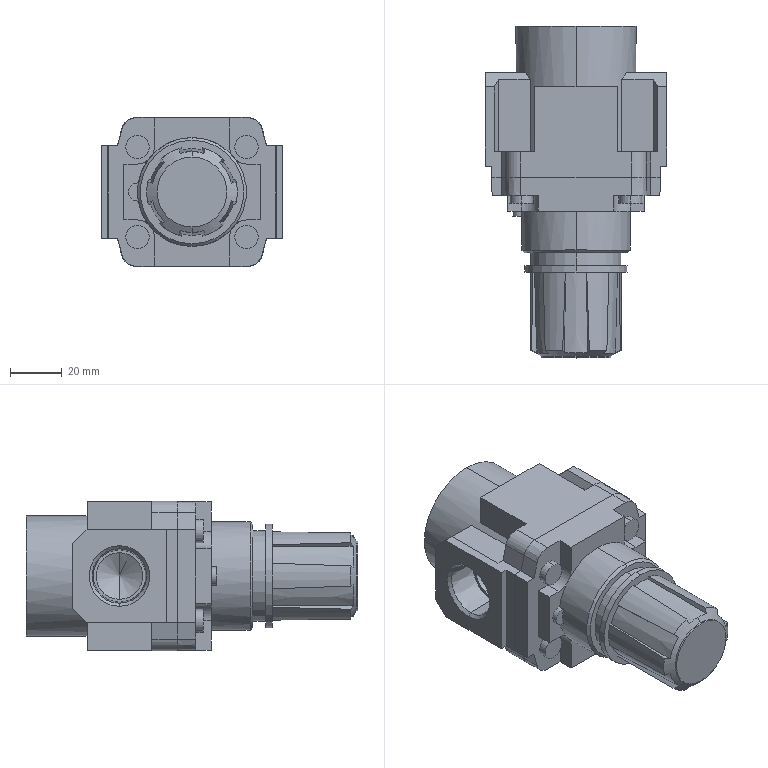Part | STEP file | AC40-04-KSTV-38JNR_AC3009A AR Body-1 | 1 solid | 172 faces | box 70 x 128 x 57.6 mm | volume 240174 mm3 | plane 103 | cylinder 39 | cone 30 | commonest cylinder face diameters 9 x8 35 x8 12 x4 13 x4 18 x4 11 x2